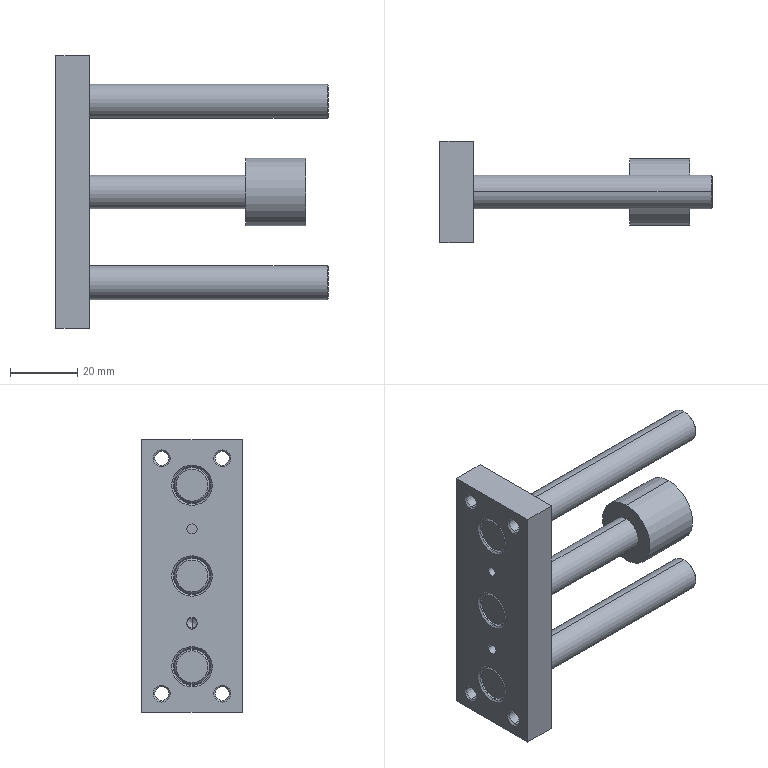Part | SolidWorks | features BaseBody 1 | 1 solid | 90 faces | box 81 x 30 x 81 mm | volume 43817 mm3 | cylinder 35 | cone 34 | plane 21 | commonest cylinder face diameters 4.134 x8 3 x7 10 x6 10.5 x6 11 x6 20 x2